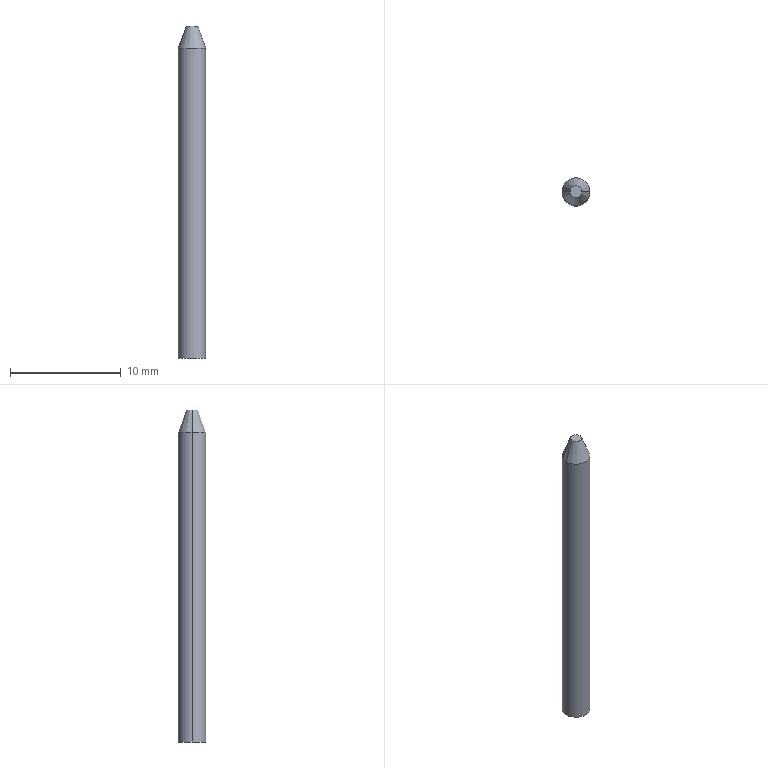Part | SolidWorks | features Chamfer 1, Extrusion 1 | 1 solid | 6 faces | box 2.5 x 2.5 x 30 mm | volume 142.655 mm3 | cone 2 | cylinder 2 | plane 2 | commonest cylinder face diameters 2.5 x2
STEP:
#1=CARTESIAN_POINT('',(0.5221,0.,30.));
#2=VERTEX_POINT('',#1);
#3=CARTESIAN_POINT('',(-0.5221,0.,30.));
#4=VERTEX_POINT('',#3);
#5=CARTESIAN_POINT('',(0.,0.,30.));
#6=DIRECTION('',(0.,0.,1.));
#7=DIRECTION('',(1.,0.,0.));
#8=AXIS2_PLACEMENT_3D('',#5,#6,#7);
#9=CIRCLE('',#8,0.5221);
#10=EDGE_CURVE('',#2,#4,#9,.T.);
#11=ORIENTED_EDGE('',*,*,#10,.F.);
#12=CARTESIAN_POINT('',(1.25,0.,28.));
#13=VERTEX_POINT('',#12);
#14=CARTESIAN_POINT('',(0.5221,0.,30.));
#15=DIRECTION('',(0.342,0.,-0.9397));
#16=VECTOR('',#15,1000.);
#17=LINE('',#14,#16);
#18=EDGE_CURVE('',#2,#13,#17,.T.);
#19=ORIENTED_EDGE('',*,*,#18,.T.);
#20=CARTESIAN_POINT('',(-1.25,0.,28.));
#21=VERTEX_POINT('',#20);
#22=CARTESIAN_POINT('',(0.,0.,28.));
#23=DIRECTION('',(0.,0.,-1.));
#24=DIRECTION('',(1.,0.,0.));
#25=AXIS2_PLACEMENT_3D('',#22,#23,#24);
#26=CIRCLE('',#25,1.25);
#27=EDGE_CURVE('',#21,#13,#26,.T.);
#28=ORIENTED_EDGE('',*,*,#27,.F.);
#29=CARTESIAN_POINT('',(-0.5221,0.,30.));
#30=DIRECTION('',(-0.342,0.,-0.9397));
#31=VECTOR('',#30,1000.);
#32=LINE('',#29,#31);
#33=EDGE_CURVE('',#4,#21,#32,.T.);
#34=ORIENTED_EDGE('',*,*,#33,.F.);
#35=EDGE_LOOP('',(#11,#19,#28,#34));
#36=FACE_OUTER_BOUND('',#35,.T.);
#37=CARTESIAN_POINT('',(0.,0.,30.));
#38=DIRECTION('',(0.,0.,-1.));
#39=DIRECTION('',(-1.,0.,0.));
#40=AXIS2_PLACEMENT_3D('',#37,#38,#39);
#41=CONICAL_SURFACE('',#40,0.5221,0.3491);
#42=ADVANCED_FACE('',(#36),#41,.T.);
#43=ORIENTED_EDGE('',*,*,#27,.T.);
#44=CARTESIAN_POINT('',(1.25,0.,0.));
#45=VERTEX_POINT('',#44);
#46=CARTESIAN_POINT('',(1.25,0.,30.));
#47=DIRECTION('',(0.,0.,-1.));
#48=VECTOR('',#47,1000.);
#49=LINE('',#46,#48);
#50=EDGE_CURVE('',#13,#45,#49,.T.);
#51=ORIENTED_EDGE('',*,*,#50,.T.);
#52=CARTESIAN_POINT('',(-1.25,0.,0.));
#53=VERTEX_POINT('',#52);
#54=CARTESIAN_POINT('',(0.,0.,0.));
#55=DIRECTION('',(0.,0.,1.));
#56=DIRECTION('',(1.,0.,0.));
#57=AXIS2_PLACEMENT_3D('',#54,#55,#56);
#58=CIRCLE('',#57,1.25);
#59=EDGE_CURVE('',#45,#53,#58,.T.);
#60=ORIENTED_EDGE('',*,*,#59,.T.);
#61=CARTESIAN_POINT('',(-1.25,0.,30.));
#62=DIRECTION('',(0.,0.,-1.));
#63=VECTOR('',#62,1000.);
#64=LINE('',#61,#63);
#65=EDGE_CURVE('',#21,#53,#64,.T.);
#66=ORIENTED_EDGE('',*,*,#65,.F.);
#67=EDGE_LOOP('',(#43,#51,#60,#66));
#68=FACE_OUTER_BOUND('',#67,.T.);
#69=CARTESIAN_POINT('',(0.,0.,30.));
#70=DIRECTION('',(0.,0.,-1.));
#71=DIRECTION('',(-1.,0.,0.));
#72=AXIS2_PLACEMENT_3D('',#69,#70,#71);
#73=CYLINDRICAL_SURFACE('',#72,1.25);
#74=ADVANCED_FACE('',(#68),#73,.T.);
#75=ORIENTED_EDGE('',*,*,#50,.F.);
#76=CARTESIAN_POINT('',(0.,0.,28.));
#77=DIRECTION('',(0.,0.,-1.));
#78=DIRECTION('',(1.,0.,0.));
#79=AXIS2_PLACEMENT_3D('',#76,#77,#78);
#80=CIRCLE('',#79,1.25);
#81=EDGE_CURVE('',#13,#21,#80,.T.);
#82=ORIENTED_EDGE('',*,*,#81,.T.);
#83=ORIENTED_EDGE('',*,*,#65,.T.);
#84=CARTESIAN_POINT('',(0.,0.,0.));
#85=DIRECTION('',(0.,0.,1.));
#86=DIRECTION('',(1.,0.,0.));
#87=AXIS2_PLACEMENT_3D('',#84,#85,#86);
#88=CIRCLE('',#87,1.25);
#89=EDGE_CURVE('',#53,#45,#88,.T.);
#90=ORIENTED_EDGE('',*,*,#89,.T.);
#91=EDGE_LOOP('',(#75,#82,#83,#90));
#92=FACE_OUTER_BOUND('',#91,.T.);
#93=CARTESIAN_POINT('',(0.,0.,30.));
#94=DIRECTION('',(0.,0.,-1.));
#95=DIRECTION('',(-1.,0.,0.));
#96=AXIS2_PLACEMENT_3D('',#93,#94,#95);
#97=CYLINDRICAL_SURFACE('',#96,1.25);
#98=ADVANCED_FACE('',(#92),#97,.T.);
#99=CARTESIAN_POINT('',(0.,0.,30.));
#100=DIRECTION('',(0.,0.,1.));
#101=DIRECTION('',(1.,0.,0.));
#102=AXIS2_PLACEMENT_3D('',#99,#100,#101);
#103=CIRCLE('',#102,0.5221);
#104=EDGE_CURVE('',#4,#2,#103,.T.);
#105=ORIENTED_EDGE('',*,*,#104,.T.);
#106=ORIENTED_EDGE('',*,*,#10,.T.);
#107=EDGE_LOOP('',(#105,#106));
#108=FACE_OUTER_BOUND('',#107,.T.);
#109=CARTESIAN_POINT('',(0.,0.,30.));
#110=DIRECTION('',(0.,0.,1.));
#111=DIRECTION('',(1.,0.,0.));
#112=AXIS2_PLACEMENT_3D('',#109,#110,#111);
#113=PLANE('',#112);
#114=ADVANCED_FACE('',(#108),#113,.T.);
#115=ORIENTED_EDGE('',*,*,#89,.F.);
#116=ORIENTED_EDGE('',*,*,#59,.F.);
#117=EDGE_LOOP('',(#115,#116));
#118=FACE_OUTER_BOUND('',#117,.T.);
#119=CARTESIAN_POINT('',(0.,0.,0.));
#120=DIRECTION('',(0.,0.,1.));
#121=DIRECTION('',(1.,0.,0.));
#122=AXIS2_PLACEMENT_3D('',#119,#120,#121);
#123=PLANE('',#122);
#124=ADVANCED_FACE('',(#118),#123,.F.);
#125=ORIENTED_EDGE('',*,*,#18,.F.);
#126=ORIENTED_EDGE('',*,*,#104,.F.);
#127=ORIENTED_EDGE('',*,*,#33,.T.);
#128=ORIENTED_EDGE('',*,*,#81,.F.);
#129=EDGE_LOOP('',(#125,#126,#127,#128));
#130=FACE_OUTER_BOUND('',#129,.T.);
#131=CARTESIAN_POINT('',(0.,0.,30.));
#132=DIRECTION('',(0.,0.,-1.));
#133=DIRECTION('',(-1.,0.,0.));
#134=AXIS2_PLACEMENT_3D('',#131,#132,#133);
#135=CONICAL_SURFACE('',#134,0.5221,0.3491);
#136=ADVANCED_FACE('',(#130),#135,.T.);
#137=CLOSED_SHELL('',(#42,#74,#98,#114,#124,#136));
#138=MANIFOLD_SOLID_BREP('',#137);
#139=CARTESIAN_POINT('',(0.,0.,0.));
#140=DIRECTION('',(0.,0.,1.));
#141=DIRECTION('',(1.,0.,0.));
#142=AXIS2_PLACEMENT_3D('',#139,#140,#141);
#143=(LENGTH_UNIT()NAMED_UNIT(*)SI_UNIT(.MILLI.,.METRE.));
#144=UNCERTAINTY_MEASURE_WITH_UNIT(LENGTH_MEASURE(0.00001),#143,'','');
#145=(NAMED_UNIT(*)PLANE_ANGLE_UNIT()SI_UNIT($,.RADIAN.));
#146=(NAMED_UNIT(*)SI_UNIT($,.STERADIAN.)SOLID_ANGLE_UNIT());
#147=(GEOMETRIC_REPRESENTATION_CONTEXT(3)GLOBAL_UNCERTAINTY_ASSIGNED_CONTEXT((#144))GLOBAL_UNIT_ASSIGNED_CONTEXT((#143,#145,#146))REPRESENTATION_CONTEXT('',''));
#148=ADVANCED_BREP_SHAPE_REPRESENTATION('',(#138,#142),#147);